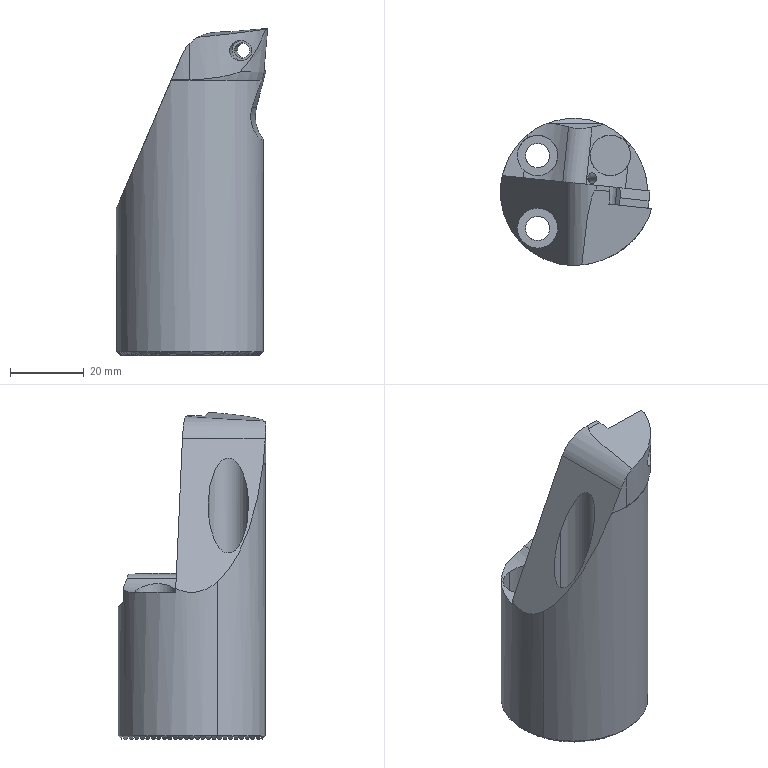NC program | Mastercam | posted with a generic post
Lines 1 to 21 of 11394:
%
:0001()
(MATERIAL - ALUMINUM MM - 2024)
(T1|12 FEMR |H1|XY STOCK TO LEAVE - .1|Z STOCK TO LEAVE - .1)
(T3|3 DR |H3)
(T4|6 FEMR |H4|XY STOCK TO LEAVE - .1|Z STOCK TO LEAVE - .1)
(T5|3 FEMR |H5|D5|WEAR COMP|TOOL DIA. - 3.|XY STOCK TO LEAVE - .05|Z STOCK TO LEAVE - .1)
(T6|12 FEMF |H6|D6|WEAR COMP|TOOL DIA. - 12.)
(T7|4 FEMF |H7|D7|WEAR COMP|TOOL DIA. - 4.)
(T8|2 XXXX |H8|D8|WEAR COMP|TOOL DIA. - 2.|XY STOCK TO LEAVE - .2|Z STOCK TO LEAVE - 0.)
(T9|30 BNOS |H9|D9|WEAR COMP|TOOL DIA. - 30.|XY STOCK TO LEAVE - .1|Z STOCK TO LEAVE - .01)
(T10|6 CHM |H10)
(T11|4.2 DR |H11)
(T12|5.5 FEM |H12)
(T14|4.05 X 0.8 THML |H14|D14|WEAR COMP|TOOL DIA. - 4.05)
(T13|2.5 BM |H13)
(T15|M6 X 1 RH |H15)
N100 G21
N102 G0 G17 G40 G80 G90 G94 G98
N104 G0 G28 G91 Z0.
N106 G0 G28 X0. Y0.